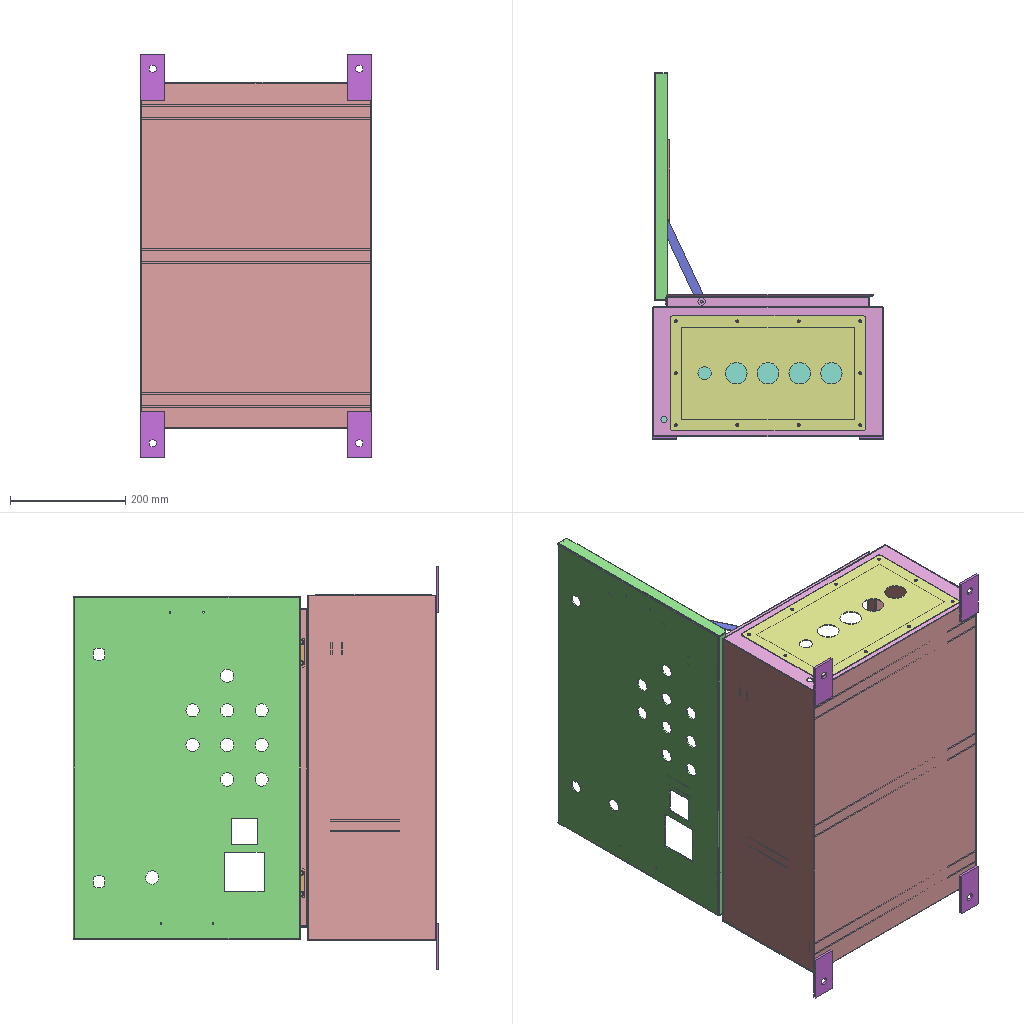Assembly | SolidWorks | 17 different items | 26 placed | box 400 x 635 x 700 mm
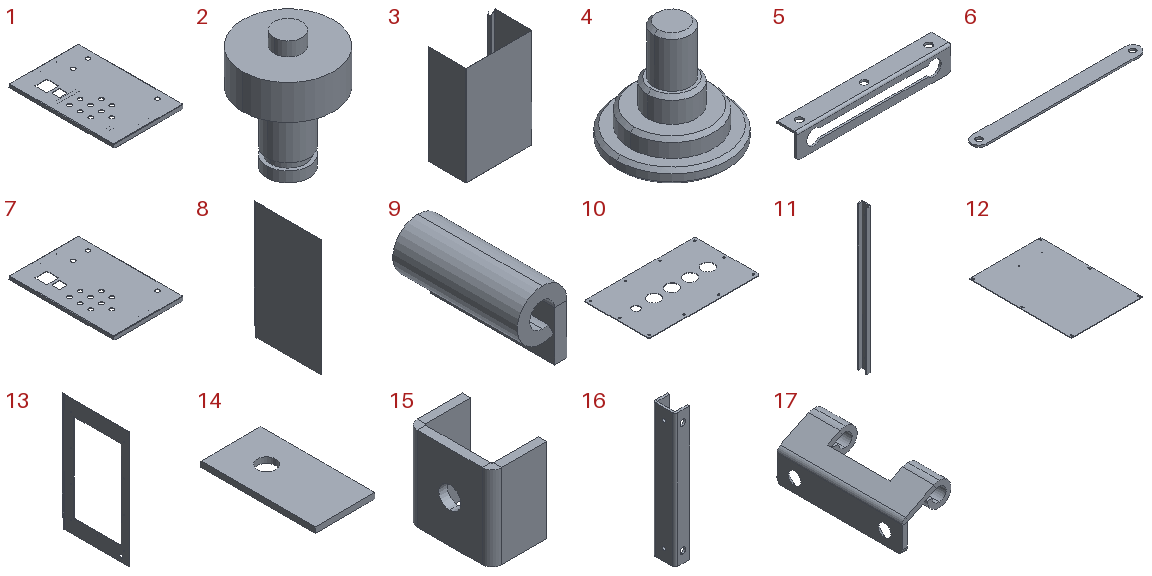Parts list (item | name | quantity | parent item | size | volume | features):
1 | (subassembly) | x1 | - | 395 x 595 x 23 mm | 532473 mm3 | -
2 | - | x1 | - | 13 x 13 x 17 mm | 962.898 mm3 | features Boss 4, Extrusion 1
3 | - | x1 | - | 400 x 247 x 600 mm | 843291 mm3 | features Cut 4, FlatPattern 1, MirrorSolid 1, SMBaseFlange 1, SheetMetal 1
4 | - | x1 | - | 16 x 16 x 15 mm | 946.808 mm3 | features Boss 3, Chamfer 1, FlatPattern 1, SMBaseFlange 1, SheetMetal 1
5 | - | x1 | - | 155 x 20 x 25 mm | 10088 mm3 | features Cut 2, Fillet 1, FlatPattern 1, SMBaseFlange 1, SheetMetal 1
6 | - | x1 | - | 175 x 15 x 2 mm | 5033 mm3 | features FlatPattern 1, SMBaseFlange 1, SheetMetal 1
7 | - | x1 | in 1 | 395 x 595 x 23 mm | 521270 mm3 | features EdgeFlange 3, Cut 1, FlatPattern 1, SMBaseFlange 1, SheetMetal 1
8 | - | x1 | - | 26 x 244.5 x 396 mm | 210973 mm3 | features Cut 2, FlatPattern 1, SMBaseFlange 1, SheetMetal 1
9 | - | x2 | - | 10 x 25 x 15 mm | 1841 mm3 | features FlatPattern 1, SMBaseFlange 1, SheetMetal 1
10 | - | x1 | - | 340 x 200 x 1.5 mm | 94399 mm3 | features FlatPattern 1, SMBaseFlange 1, SheetMetal 1
11 | - | x3 | - | 13 x 25 x 395 mm | 44005 mm3 | features Cut 1, FlatPattern 1, SMBaseFlange 1, SheetMetal 1
12 | - | x1 | - | 360 x 520 x 2.5 mm | 466582 mm3 | features FlatPattern 1, SMBaseFlange 1, SheetMetal 1
13 | - | x1 | - | 25.5 x 245.5 x 397 mm | 87187 mm3 | features Cut 4, FlatPattern 1, SMBaseFlange 1, SheetMetal 1
14 | - | x4 | - | 42 x 80 x 4 mm | 12909 mm3 | features FlatPattern 1, SMBaseFlange 1, SheetMetal 1
15 | - | x2 | in 1 | 13 x 20 x 20 mm | 1593 mm3 | features Cut 1, FlatPattern 1, SMBaseFlange 1, SheetMetal 1
16 | - | x2 | in 1 | 13 x 20 x 120 mm | 9610 mm3 | features Cut 2, FlatPattern 1, SMBaseFlange 1, SheetMetal 1
17 | - | x2 | - | 19.5 x 50 x 18.659 mm | 2993 mm3 | features Cut 2, Chamfer 1, Fillet 1, FlatPattern 1, SMBaseFlange 1, SheetMetal 1
Mates (type | each side: item.copy, entity, surface, feature):
In the top assembly
Coincident | 3.1 face plane Base-Flange1 | 11.1 face plane Base-Flange1
DistanceDim | 3.1 face plane Base-Flange1 | 11.1 face plane Base-Flange1
DistanceDim | 3.1 face plane Mirror1 | 11.1 face plane Base-Flange1
Coincident | 11.1 face plane Base-Flange1 | 12.1 face plane Base-Flange1
DistanceDim | 3.1 face plane Base-Flange1 | 12.1 face plane Base-Flange1 | 2 times
Coincident | 3.1 face plane Mirror1 | 13.1 face plane Base-Flange1 | 3 times
Coincident | 3.1 face plane Mirror1 | 8.1 face plane Base-Flange1 | 2 times
Coincident | 3.1 face plane Base-Flange1 | 8.1 face plane Base-Flange1
Coincident | 3.1 face plane Base-Flange1 | 17.1 face plane Base-Flange1
Concentric | 3.1 edge | 17.1 edge | 2 times
Coincident | 3.1 face plane Base-Flange1 | 17.2 face plane Base-Flange1
Concentric | 3.1 edge | 17.2 edge | 2 times
Concentric | 17.2 edge | 9.1 edge
Coincident | 17.2 face plane Cut-Extrude1 | 9.1 face plane Base-Bend1
Concentric | 17.1 edge | 9.2 edge
Coincident | 17.1 face plane Cut-Extrude1 | 9.2 face plane Base-Bend1
Coincident | 9.1 face plane Base-Flange1 | 7.1 face plane Edge-Flange3
Coincident | 9.2 face plane Base-Flange1 | 7.1 face plane Edge-Flange3
Tangent | 9.1 face cylinder Base-Bend1 | 7.1 face plane Base-Flange1
DistanceDim | 13.1 face plane Base-Flange1 | 7.1 face plane Edge-Flange1
Coincident | 3.1 face plane Base-Flange1 | 15.1 face plane Base-Flange1
DistanceDim | 3.1 face plane Base-Flange1 | 15.1 face plane Base-Flange1
Coincident | 15.2 face plane Base-Flange1 | 15.1 face plane Base-Flange1
Coincident | 13.1 face plane Base-Flange1 | 10.1 face plane Base-Flange1
Concentric | 13.1 edge | 10.1 edge | 2 times
Coincident | 3.1 face plane Base-Flange1 | 14.1 face plane Base-Flange1 | 2 times
Coincident | 14.1 face plane Base-Flange1 | 14.2 face plane Base-Flange1
Coincident | 14.2 face plane Base-Flange1 | 14.3 face plane Base-Flange1
Coincident | 14.4 face plane Base-Flange1 | 14.2 face plane Base-Flange1 | 2 times
DistanceDim | 8.1 face plane Base-Flange1 | 14.1 face plane Base-Flange1
Coincident | 3.1 face plane Mirror1 | 14.3 face plane Base-Flange1
Coincident | 14.1 face plane Base-Flange1 | 14.3 face plane Base-Flange1
Coincident | 3.1 face plane Base-Flange1 | 14.2 face plane Base-Flange1
DistanceDim | 13.1 face plane Base-Flange1 | 14.2 face plane Base-Flange1
Coincident | 3.1 face plane Mirror1 | 14.4 face plane Base-Flange1
Coincident | 15.1 face plane Base-Flange1 | 16.1 face plane Base-Flange1
Concentric | 13.1 face cylinder Cut-Extrude4 | 2.1 face cylinder Extrude3
Coincident | 13.1 face plane Base-Flange1 | 2.1 face plane Extrude1
Coincident | 7.1 face plane Base-Flange1 | 5.1 face plane Base-Flange1
DistanceDim | 7.1 face plane Edge-Flange1 | 5.1 face plane Base-Flange1
DistanceDim | 7.1 face plane Edge-Flange3 | 5.1 face plane Base-Flange1
Concentric | 2.1 face cylinder Extrude3 | 6.1 edge
DistanceDim | 5.1 face plane Base-Flange1 | 6.1 face plane Base-Flange1
Concentric | 6.1 face cylinder Base-Flange1 | 4.1 face cylinder Extrude3
DistanceDim | 5.1 face plane Base-Flange1 | 4.1 face plane Extrude1
DistanceDim | 5.1 face plane Cut-Extrude2 | 4.1 face cylinder Extrude2
DistanceDim | 8.1 face plane Base-Flange1 | 16.1 face plane Base-Flange1 | 2 times
Parallel | 3.1 face plane Base-Flange1 | 7.1 face plane Base-Flange1
In subassembly 1
Coincident | 7.2 face plane Base-Flange1 | 16.1 face plane Base-Flange1
Coincident | 7.2 face plane Base-Flange1 | 15.1 face plane Base-Flange1
DistanceDim | 7.2 face plane Edge-Flange3 | 15.1 face plane Base-Flange1
DistanceDim | 7.2 face plane Edge-Flange1 | 15.1 face plane Base-Flange1
DistanceDim | 7.2 face plane Edge-Flange3 | 16.1 face plane Base-Flange1
DistanceDim | 7.2 face plane Base-Flange1 | 16.1 face plane Base-Flange1